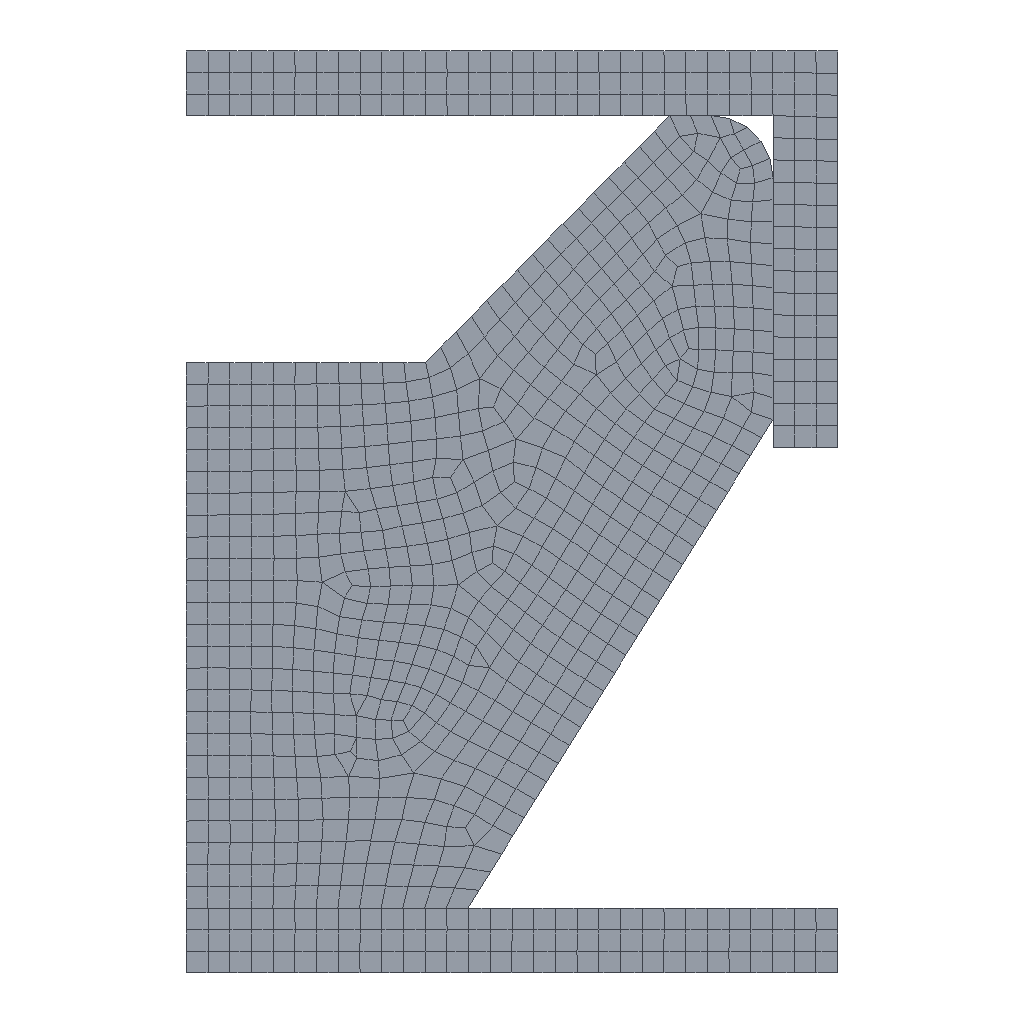Simulation study | ansys workbench
Set-up summary:
category,name,step,type,value,unit,region
solver,ansys_workbench
units,mm-N-s-tonne (MPa),,stated,"/units,MPA"
analysis,LS1,,static
load_step,LS1,LS1,static,nsubst=5; time=1
mesh,nodes,,,2949
mesh,elements,,,1186
element_type,PLANE183,,,894
element_type,TARGE169,,,146
element_type,CONTA172,,,146
material,Structural Steel,,E,200000,tonne s^-2 mm^-1
material,Structural Steel,,nu,0.3
material,Structural Steel,,density,7.85e-09,tonne mm^-3
material,Structural Steel,,conductivity,60.5,tonne mm s^-3 C^-1
material,Structural Steel,,specific_heat,4.34e+08,mm^2 s^-2 C^-1
material,Structural Steel,,cte,1.2e-05,C^-1
material,Structural Steel,,permeability,10000
material,Structural Steel,,resistivity,0.00017,ohm mm
material,?,,behaviors,"hyperelastic; tb hype,YEOH"
bc,Fixed Supports,model,fixed,[dofs=ALL],,_FIXEDSU
bc,Constant Zero Displacement X,model,fixed,[dofs=UX],,_DISPZEROUX
bc,Set Displacements,LS1,prescribed uy,-15 [dofs=UY],,_CM50UY_YP
contact,Frictional - ______|NONE ? ____|NONE,,standard (frictionless/frictional),friction=0.8; element=CONTA172
contact,Frictional - ______-0|NONE ? ____|NONE,,standard (frictionless/frictional),friction=0.5; element=CONTA172
named_set,_FIXEDSU,,node,337
named_set,_DISPZEROUX,,node,502
named_set,_CM50UY_YP,,node,502
Ansys APDL input file, long lists of numbers shortened:
/batch
/config,noeldb,1     ! force off writing results to database
*get,_wallstrt,active,,time,wall
! ANSYS input file written by Workbench version 2021 R1
! File used for geometry attach:
/title,_____--____ (A5)
! ****** Begin Custom Load Command Snippet ******
/COM, ACT Extensions:
/COM,     LSDYNA, 2021.1
/COM,
! ****** End   Custom Load Command Snippet ******
*DIM,_wb_ProjectScratch_dir,string,248
_wb_ProjectScratch_dir(1) = ''
*DIM,_wb_SolverFiles_dir,string,248
_wb_SolverFiles_dir(1) = ''
*DIM,_wb_userfiles_dir,string,248
_wb_userfiles_dir(1) = ''
/com,--- Data in consistent NMM units. See Solving Units in the help system for more information.
/units,MPA
/nopr
/wb,file,start              !  signify a WB generated input file
/prep7
! Turn off shape checking because checks already performed inside WB mesher.
! See help system for more information.
SHPP,OFF,,NOWARN
/nolist
etcon,set             ! allow ANSYS to choose best KEYOP's for 180x elements, resets any applicable keyopt to MAPDL defaults
/com,*********** Nodes for the whole assembly ***********
nblock,3,,3243
(1i9,3e20.9e3)
        1     0.000000000E+00     1.500000000E+01     0.000000000E+00
! (2948 more lines like these left out)
-1
/wb,elem,start            !  set before creation of elements
/com,*********** Elements for Body 1 "______|NONE" ***********
et,1,183
keyo,1,3,1
eblock,19,solid,,90
(19i9)
        1        1        1        1        0        0        0        0        8        0        1       67       34        5       36      190      132      133      194
! (89 more lines like these left out)
-1
/com,*********** Elements for Body 2 "______-0|NONE" ***********
et,2,183
keyo,2,3,1
eblock,19,solid,,135
(19i9)
        2        2        2        2        0        0        0        0        8        0       91      434      450      449      521      711      740      742      712
! (134 more lines like these left out)
-1
/com,*********** Elements for Body 3 "____|NONE" ***********
et,3,183
keyo,3,3,1
eblock,19,solid,,669
(19i9)
        3        3        3        3        0        0        0        0        8        0      226     1290      895      896      896     1672     1671      896     1673
! (668 more lines like these left out)
-1
/wb,elem,end               !  done creating elements
/com,*********** Send User Defined Coordinate System(s) ***********
csys,0
toffst,273.15,  ! Temperature offset from absolute zero
/com,*********** Set Reference Temperature ***********
tref,22.
/wb,mat,start              !  starting to send materials
/com,*********** Send Materials ***********
Temperature = 'TEMP' ! Temperature
MP,DENS,1,7.85e-09,	! tonne mm^-3
MP,ALPX,1,1.2e-05,	! C^-1
MP,C,1,434000000,	! mm^2 s^-2 C^-1
MP,KXX,1,60.5,	! tonne mm s^-3 C^-1
MP,RSVX,1,0.00017,	! ohm mm
MP,EX,1,200000,	! tonne s^-2 mm^-1
MP,NUXY,1,0.3,
MP,MURX,1,10000,
Temperature = 'TEMP' ! Temperature
MP,DENS,2,7.85e-09,	! tonne mm^-3
MP,ALPX,2,1.2e-05,	! C^-1
MP,C,2,434000000,	! mm^2 s^-2 C^-1
MP,KXX,2,60.5,	! tonne mm s^-3 C^-1
MP,RSVX,2,0.00017,	! ohm mm
MP,EX,2,200000,	! tonne s^-2 mm^-1
MP,NUXY,2,0.3,
MP,MURX,2,10000,
TB,HYPE,3,1,3,YEOH
TBDATA,1,2.2,0.8,0.01,0.001,0.001,0.001
/wb,mat,end                !  done sending materials
/com,*********** Send Sheet Properties ***********
!************************* Model Summary ********************
!______|NONE,	结构钢,	matid,	1
!______-0|NONE,	结构钢,	matid,	2
!____|NONE,	超弹性橡胶,	matid,	3
!************************* End Model Summary ********************
! get the diagonal of the bounding box. Needed later for other things
*get,_xmin,node,,mnloc,x
*get,_ymin,node,,mnloc,y
*get,_zmin,node,,mnloc,z
*get,_xmax,node,,mxloc,x
*get,_ymax,node,,mxloc,y
*get,_zmax,node,,mxloc,z
_ASMDIAG=(_xmax-_xmin)*(_xmax-_xmin)+(_ymax-_ymin)*(_ymax-_ymin)+(_zmax-_zmin)*(_zmax-_zmin)
_ASMDIAG=SQRT(_ASMDIAG)
/wb,contact,start          !  starting to send contact
/com,*********** Create Contact "摩擦的 - ______|NONE 至 ____|NONE" ***********
/com,            Real Constant Set For Above Contact Is 5 & 4
*set,tid,5
*set,cid,4
r,tid
r,cid
et,tid,169
et,cid,172
eblock,10,,,30
(15i9)
      895        5        5        5        0       66        1      126
! (29 more lines like these left out)
-1
eblock,10,,,30
(15i9)
      925        4        4        4        0       66        1      126
! (29 more lines like these left out)
-1
eblock,10,,,40
(15i9)
      955        4        5        4        0      853      841     1563
! (39 more lines like these left out)
-1
eblock,10,,,40
(15i9)
      995        5        4        5        0      853      841     1563
! (39 more lines like these left out)
-1
keyo,cid,8,2               ! auto create asymmetric contact (from Program Controlled setting)
keyo,cid,10,0              ! adjust contact stiffness each NR iteration (from Program Controlled setting)
keyo,cid,12,0              ! standard contact
mp,mu,cid,0.8       ! unitless
keyo,cid,2,0               ! augmented Lagrange (from Program Controlled setting)
keyo,cid,4,0               ! on Gauss point (from Program Controlled setting)
keyo,cid,9,0               ! use real geometry with stepped effects
keyo,cid,7,0               ! No Prediction
rmod,tid,3,1.       ! FKN
rmod,tid,5,0.       ! ICONT
rmod,tid,6,-0.6548  ! PINB
rmod,tid,10,0.      ! CNOF
rmod,tid,12,0.      ! FKT
rmod,tid,36,37      ! WB DSID
rmod,cid,3,1.       ! FKN
rmod,cid,5,0.       ! ICONT
rmod,cid,6,-0.6548  ! PINB
rmod,cid,10,0.      ! CNOF
rmod,cid,12,0.      ! FKT
rmod,cid,36,37      ! WB DSID
/com,*********** Create Contact "摩擦的 - ______-0|NONE 至 ____|NONE" ***********
/com,            Real Constant Set For Above Contact Is 7 & 6
*set,tid,7
*set,cid,6
r,tid
r,cid
et,tid,169
et,cid,172
eblock,10,,,42
(15i9)
     1035        7        7        7        0      419      393      628
! (41 more lines like these left out)
-1
eblock,10,,,42
(15i9)
     1077        6        6        6        0      419      393      628
! (41 more lines like these left out)
-1
eblock,10,,,34
(15i9)
     1119        6        7        6        0      895      896     1671
! (33 more lines like these left out)
-1
eblock,10,,,34
(15i9)
     1153        7        6        7        0      895      896     1671
! (33 more lines like these left out)
-1
keyo,cid,8,2               ! auto create asymmetric contact (from Program Controlled setting)
keyo,cid,10,0              ! adjust contact stiffness each NR iteration (from Program Controlled setting)
keyo,cid,12,0              ! standard contact
mp,mu,cid,0.5       ! unitless
keyo,cid,2,0               ! augmented Lagrange (from Program Controlled setting)
keyo,cid,4,0               ! on Gauss point (from Program Controlled setting)
keyo,cid,9,0               ! use real geometry with stepped effects
keyo,cid,7,0               ! No Prediction
rmod,tid,3,1.       ! FKN
rmod,tid,5,0.       ! ICONT
rmod,tid,6,-0.6548  ! PINB
rmod,tid,10,0.      ! CNOF
rmod,tid,12,0.      ! FKT
rmod,tid,36,40      ! WB DSID
rmod,cid,3,1.       ! FKN
rmod,cid,5,0.       ! ICONT
rmod,cid,6,-0.6548  ! PINB
rmod,cid,10,0.      ! CNOF
rmod,cid,12,0.      ! FKT
rmod,cid,36,40      ! WB DSID
nsel,all
esel,all
/wb,contact,end            !  done creating contacts
/golist
/wb,load,start             !  starting to send loads
/com,*********** Fixed Supports ***********
CMBLOCK,_FIXEDSU,NODE,      337
(8i10)
         1         2         3         4         5         6         7         8
! (42 more lines like these left out)
cmsel,s,_FIXEDSU
d,all,all
nsel,all
/com,******* Constant Zero Displacement X *******
CMBLOCK,_DISPZEROUX,NODE,      502
(8i10)
       338       339       340       341       342       343       344       345
! (62 more lines like these left out)
cmsel,s,_DISPZEROUX
d,all,ux,0
nsel,all
/gst,on,on
fini
*get,_numnode,node,0,count
*get,_numelem,elem,0,count
*get, _MAXELEMNUM, elem, 0, NUM, MAX
*get, _MAXNODENUM, node, 0, NUM, MAX
*get, _MAXELEMTYPE, etyp, 0, NUM, MAX
*get, _MAXREALCONST, real, 0, NUM, MAX
/go
/wb,load,end               !  done creating loads
/com,--- Number of total nodes = %_numnode%
/com,--- Number of contact elements = 292
/com,--- Number of spring elements = 0
/com,--- Number of bearing elements = 0
/com,--- Number of solid elements = 894
/com,--- Number of condensed parts = 0
/com,--- Number of total elements = %_numelem%
*get,_wallbsol,active,,time,wall
/com,****************************************************************************
/com,*************************    SOLUTION       ********************************
/com,****************************************************************************
/solu
antype,0                   ! static analysis
nlgeom,on                  ! Turn on Large Deformation Effects
_thickRatio=  0     ! Ratio of thick parts in the model
eqsl,sparse,,,,,1
cntr,print,1               ! print out contact info and also make no initial contact an error
dmpoption,emat,no             ! Don't combine emat file for DANSYS
dmpoption,esav,no             ! Don't combine esav file for DANSYS
nldiag,cont,iter           ! print out contact info each equilibrium iteration
rescontrol,define,last,last,,dele	   ! Program Controlled
/com,****************************************************
/com,******************* SOLVE FOR LS 1 OF 1 ****************
/com,*** Set Displacements ***
CMBLOCK,_CM50UY_YP,NODE,      502
(8i10)
       338       339       340       341       342       343       344       345
! (62 more lines like these left out)
cmsel,s,_CM50UY_YP
d,all,uy,-15.
nsel,all
/com,*** Component For All Non-Zero UY Displacements ***
cmsel,s,_CM50uy_yp
cm,_DISPNONZEROUY,NODE
nsel,all
/nopr
/gopr
/nolist
autots,on                  ! Workbench Program Controlled automatic time stepping
nsub,5,1000,1              ! due to presence of nonlinear materials
time,1.
outres,erase
outres,all,none
outres,nsol,all,
outres,rsol,all
outres,eangl,all
outres,etmp,all
outres,veng,all
outres,strs,all,
outres,epel,all,
outres,eppl,all,
outres,cont,all,
! *********** WB SOLVE COMMAND ***********
! check interactive state
*get,ANSINTER_,active,,int
*if,ANSINTER_,ne,0,then
/eof
*endif
solve
/com *************** Write FE CONNECTORS *********
CEWRITE,file,ce,,INTE
/com,****************************************************
/com,*************** FINISHED SOLVE FOR LS 1 *************
*get,_wallasol,active,,time,wall
/nopr
*get,_numnode,node,0,count
*get,_numelem,elem,0,count
*get, _MAXELEMNUM, elem, 0, NUM, MAX
*get, _MAXNODENUM, node, 0, NUM, MAX,,,INTERNAL
*get, _MAXELEMTYPE, etyp, 0, NUM, MAX
*get, _MAXREALCONST, real, 0, NUM, MAX
/gopr
/post1
xmlo,ENCODING,ISO-8859-1
xmlo,parm
/xml,parm,xml
fini
/gopr
*get,_walldone,active,,time,wall
_preptime=(_wallbsol-_wallstrt)*3600
_solvtime=(_wallasol-_wallbsol)*3600
_posttime=(_walldone-_wallasol)*3600
_totaltim=(_walldone-_wallstrt)*3600
*get,_dlbratio,active,0,solu,dlbr
*get,_combtime,active,0,solu,comb
/com,--- Total number of nodes = %_numnode%
/com,--- Total number of elements = %_numelem%
/com,--- Element load balance ratio = %_dlbratio%
/com,--- Time to combine distributed files = %_combtime%
/wb,file,end               ! done with WB generated input
Results summary:
result,analyses[0].index,,,1
result,analyses[0].system,,,SYS
result,analyses[0].deck,,,deck.dat
result,analyses[0].solve_status,,,completed
result,analyses[0].analysis_type,,,static
result,analyses[0].physics,,,mechanical
result,analyses[0].unit_system,,,"NMM: mm, ton, N, s, mV, mA, degC"
result,analyses[0].n_sets,,,9
result,analyses[0].load_steps[0].set,set=9,,9
result,analyses[0].load_steps[0].time_or_freq,set=9,,1
result,analyses[0].load_steps[0].max_displacement_magnitude,set=9,,15
result,analyses[0].load_steps[0].max_von_mises_nodal,set=9,,2.409
result,analyses[0].load_steps[0].reaction_force_sum_xyz[1],set=9,,-54515.2
result,analyses[0].load_steps[0].reaction_force_sum_xyz[2],set=9,,4.417
result,analyses[0].load_steps[0].reaction_force_sum_xyz[3],set=9,,0
result,geometry_export[0][0],,,.step
result,geometry_export[0][1],,,ok
result,geometry_export[0][2],,,3